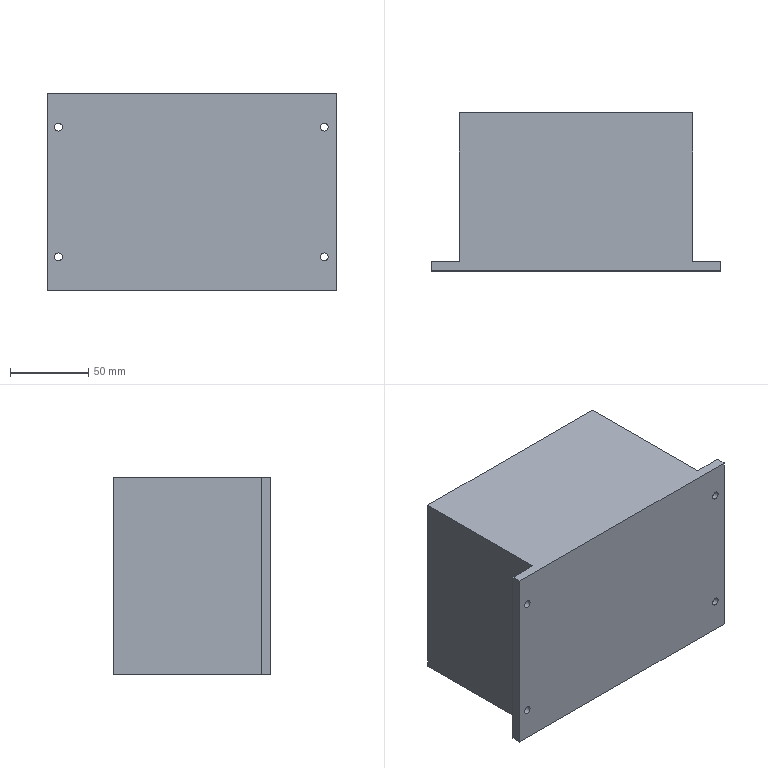Part | STEP file | Inverter | 1 solid | 14 faces | box 185 x 101 x 126 mm | volume 1922919 mm3 | plane 10 | cylinder 4 | commonest cylinder face diameters 5 x4
STEP:
#1=CARTESIAN_POINT('',(0.,0.,0.));
#2=DIRECTION('',(0.,0.,1.));
#3=DIRECTION('',(1.,0.,0.));
#4=AXIS2_PLACEMENT_3D('',#1,#2,#3);
#5=CARTESIAN_POINT('',(-110.145,6.,92.15));
#6=VERTEX_POINT('',#5);
#7=CARTESIAN_POINT('',(-110.145,0.,92.15));
#8=VERTEX_POINT('',#7);
#9=CARTESIAN_POINT('',(-110.145,101.,92.15));
#10=DIRECTION('',(0.,-1.,0.));
#11=VECTOR('',#10,1.);
#12=LINE('',#9,#11);
#13=CARTESIAN_POINT('',(-110.145,101.,-33.85));
#14=DIRECTION('',(1.,0.,0.));
#15=DIRECTION('',(0.,0.,-1.));
#16=AXIS2_PLACEMENT_3D('',#13,#14,#15);
#17=PLANE('',#16);
#18=CARTESIAN_POINT('',(-126.,0.));
#19=DIRECTION('',(0.,-1.));
#20=VECTOR('',#19,1.);
#21=LINE('',#18,#20);
#22=(GEOMETRIC_REPRESENTATION_CONTEXT(2)PARAMETRIC_REPRESENTATION_CONTEXT()REPRESENTATION_CONTEXT('',''));
#23=DEFINITIONAL_REPRESENTATION('',(#21),#22);
#24=PCURVE('',#17,#23);
#25=CARTESIAN_POINT('',(-110.145,101.,92.15));
#26=DIRECTION('',(0.,0.,-1.));
#27=DIRECTION('',(-1.,0.,0.));
#28=AXIS2_PLACEMENT_3D('',#25,#26,#27);
#29=PLANE('',#28);
#30=CARTESIAN_POINT('',(0.,0.));
#31=DIRECTION('',(0.,-1.));
#32=VECTOR('',#31,1.);
#33=LINE('',#30,#32);
#34=(GEOMETRIC_REPRESENTATION_CONTEXT(2)PARAMETRIC_REPRESENTATION_CONTEXT()REPRESENTATION_CONTEXT('',''));
#35=DEFINITIONAL_REPRESENTATION('',(#33),#34);
#36=PCURVE('',#29,#35);
#37=SURFACE_CURVE('',#12,(#24,#36),.PCURVE_S1.);
#38=EDGE_CURVE('',#6,#8,#37,.T.);
#39=ORIENTED_EDGE('',*,*,#38,.F.);
#40=CARTESIAN_POINT('',(-110.145,6.,-33.85));
#41=VERTEX_POINT('',#40);
#42=CARTESIAN_POINT('',(-110.145,6.,-33.85));
#43=DIRECTION('',(0.,0.,-1.));
#44=VECTOR('',#43,1.);
#45=LINE('',#42,#44);
#46=CARTESIAN_POINT('',(0.,-95.));
#47=DIRECTION('',(1.,0.));
#48=VECTOR('',#47,1.);
#49=LINE('',#46,#48);
#50=(GEOMETRIC_REPRESENTATION_CONTEXT(2)PARAMETRIC_REPRESENTATION_CONTEXT()REPRESENTATION_CONTEXT('',''));
#51=DEFINITIONAL_REPRESENTATION('',(#49),#50);
#52=PCURVE('',#17,#51);
#53=CARTESIAN_POINT('',(-116.411,6.,-33.85));
#54=DIRECTION('',(0.,-1.,0.));
#55=DIRECTION('',(0.,0.,-1.));
#56=AXIS2_PLACEMENT_3D('',#53,#54,#55);
#57=PLANE('',#56);
#58=CARTESIAN_POINT('',(0.,6.266));
#59=DIRECTION('',(1.,0.));
#60=VECTOR('',#59,1.);
#61=LINE('',#58,#60);
#62=(GEOMETRIC_REPRESENTATION_CONTEXT(2)PARAMETRIC_REPRESENTATION_CONTEXT()REPRESENTATION_CONTEXT('',''));
#63=DEFINITIONAL_REPRESENTATION('',(#61),#62);
#64=PCURVE('',#57,#63);
#65=SURFACE_CURVE('',#45,(#52,#64),.PCURVE_S1.);
#66=EDGE_CURVE('',#6,#41,#65,.T.);
#67=ORIENTED_EDGE('',*,*,#66,.T.);
#68=CARTESIAN_POINT('',(-110.145,0.,-33.85));
#69=VERTEX_POINT('',#68);
#70=CARTESIAN_POINT('',(-110.145,101.,-33.85));
#71=DIRECTION('',(0.,-1.,0.));
#72=VECTOR('',#71,1.);
#73=LINE('',#70,#72);
#74=CARTESIAN_POINT('',(0.,0.));
#75=DIRECTION('',(0.,-1.));
#76=VECTOR('',#75,1.);
#77=LINE('',#74,#76);
#78=(GEOMETRIC_REPRESENTATION_CONTEXT(2)PARAMETRIC_REPRESENTATION_CONTEXT()REPRESENTATION_CONTEXT('',''));
#79=DEFINITIONAL_REPRESENTATION('',(#77),#78);
#80=PCURVE('',#17,#79);
#81=CARTESIAN_POINT('',(-110.145,101.,-33.85));
#82=DIRECTION('',(0.,0.,1.));
#83=DIRECTION('',(1.,0.,0.));
#84=AXIS2_PLACEMENT_3D('',#81,#82,#83);
#85=PLANE('',#84);
#86=CARTESIAN_POINT('',(0.,0.));
#87=DIRECTION('',(0.,-1.));
#88=VECTOR('',#87,1.);
#89=LINE('',#86,#88);
#90=(GEOMETRIC_REPRESENTATION_CONTEXT(2)PARAMETRIC_REPRESENTATION_CONTEXT()REPRESENTATION_CONTEXT('',''));
#91=DEFINITIONAL_REPRESENTATION('',(#89),#90);
#92=PCURVE('',#85,#91);
#93=SURFACE_CURVE('',#73,(#80,#92),.PCURVE_S1.);
#94=EDGE_CURVE('',#41,#69,#93,.T.);
#95=ORIENTED_EDGE('',*,*,#94,.T.);
#96=CARTESIAN_POINT('',(-110.145,0.,-33.85));
#97=DIRECTION('',(0.,0.,1.));
#98=VECTOR('',#97,1.);
#99=LINE('',#96,#98);
#100=CARTESIAN_POINT('',(0.,-101.));
#101=DIRECTION('',(-1.,0.));
#102=VECTOR('',#101,1.);
#103=LINE('',#100,#102);
#104=(GEOMETRIC_REPRESENTATION_CONTEXT(2)PARAMETRIC_REPRESENTATION_CONTEXT()REPRESENTATION_CONTEXT('',''));
#105=DEFINITIONAL_REPRESENTATION('',(#103),#104);
#106=PCURVE('',#17,#105);
#107=CARTESIAN_POINT('',(0.,0.,0.));
#108=DIRECTION('',(0.,1.,0.));
#109=DIRECTION('',(0.,0.,1.));
#110=AXIS2_PLACEMENT_3D('',#107,#108,#109);
#111=PLANE('',#110);
#112=CARTESIAN_POINT('',(-33.85,-110.145));
#113=DIRECTION('',(1.,0.));
#114=VECTOR('',#113,1.);
#115=LINE('',#112,#114);
#116=(GEOMETRIC_REPRESENTATION_CONTEXT(2)PARAMETRIC_REPRESENTATION_CONTEXT()REPRESENTATION_CONTEXT('',''));
#117=DEFINITIONAL_REPRESENTATION('',(#115),#116);
#118=PCURVE('',#111,#117);
#119=SURFACE_CURVE('',#99,(#106,#118),.PCURVE_S1.);
#120=EDGE_CURVE('',#69,#8,#119,.T.);
#121=ORIENTED_EDGE('',*,*,#120,.T.);
#122=EDGE_LOOP('',(#39,#67,#95,#121));
#123=FACE_BOUND('',#122,.T.);
#124=ADVANCED_FACE('',(#123),#17,.F.);
#125=CARTESIAN_POINT('',(74.855,6.,92.15));
#126=VERTEX_POINT('',#125);
#127=CARTESIAN_POINT('',(74.855,0.,92.15));
#128=VERTEX_POINT('',#127);
#129=CARTESIAN_POINT('',(74.855,101.,92.15));
#130=DIRECTION('',(0.,-1.,0.));
#131=VECTOR('',#130,1.);
#132=LINE('',#129,#131);
#133=CARTESIAN_POINT('',(-185.,0.));
#134=DIRECTION('',(0.,-1.));
#135=VECTOR('',#134,1.);
#136=LINE('',#133,#135);
#137=(GEOMETRIC_REPRESENTATION_CONTEXT(2)PARAMETRIC_REPRESENTATION_CONTEXT()REPRESENTATION_CONTEXT('',''));
#138=DEFINITIONAL_REPRESENTATION('',(#136),#137);
#139=PCURVE('',#29,#138);
#140=CARTESIAN_POINT('',(74.855,101.,-33.85));
#141=DIRECTION('',(-1.,0.,0.));
#142=DIRECTION('',(0.,0.,1.));
#143=AXIS2_PLACEMENT_3D('',#140,#141,#142);
#144=PLANE('',#143);
#145=CARTESIAN_POINT('',(126.,0.));
#146=DIRECTION('',(0.,-1.));
#147=VECTOR('',#146,1.);
#148=LINE('',#145,#147);
#149=(GEOMETRIC_REPRESENTATION_CONTEXT(2)PARAMETRIC_REPRESENTATION_CONTEXT()REPRESENTATION_CONTEXT('',''));
#150=DEFINITIONAL_REPRESENTATION('',(#148),#149);
#151=PCURVE('',#144,#150);
#152=SURFACE_CURVE('',#132,(#139,#151),.PCURVE_S1.);
#153=EDGE_CURVE('',#126,#128,#152,.T.);
#154=ORIENTED_EDGE('',*,*,#153,.F.);
#155=CARTESIAN_POINT('',(56.855,6.,92.15));
#156=VERTEX_POINT('',#155);
#157=CARTESIAN_POINT('',(76.853,6.,92.15));
#158=DIRECTION('',(1.,0.,0.));
#159=VECTOR('',#158,1.);
#160=LINE('',#157,#159);
#161=CARTESIAN_POINT('',(-186.998,-95.));
#162=DIRECTION('',(-1.,0.));
#163=VECTOR('',#162,1.);
#164=LINE('',#161,#163);
#165=(GEOMETRIC_REPRESENTATION_CONTEXT(2)PARAMETRIC_REPRESENTATION_CONTEXT()REPRESENTATION_CONTEXT('',''));
#166=DEFINITIONAL_REPRESENTATION('',(#164),#165);
#167=PCURVE('',#29,#166);
#168=CARTESIAN_POINT('',(76.853,6.,-33.85));
#169=DIRECTION('',(0.,-1.,0.));
#170=DIRECTION('',(1.,0.,0.));
#171=AXIS2_PLACEMENT_3D('',#168,#169,#170);
#172=PLANE('',#171);
#173=CARTESIAN_POINT('',(0.,126.));
#174=DIRECTION('',(1.,0.));
#175=VECTOR('',#174,1.);
#176=LINE('',#173,#175);
#177=(GEOMETRIC_REPRESENTATION_CONTEXT(2)PARAMETRIC_REPRESENTATION_CONTEXT()REPRESENTATION_CONTEXT('',''));
#178=DEFINITIONAL_REPRESENTATION('',(#176),#177);
#179=PCURVE('',#172,#178);
#180=SURFACE_CURVE('',#160,(#167,#179),.PCURVE_S1.);
#181=EDGE_CURVE('',#156,#126,#180,.T.);
#182=ORIENTED_EDGE('',*,*,#181,.F.);
#183=CARTESIAN_POINT('',(56.855,101.,92.15));
#184=VERTEX_POINT('',#183);
#185=CARTESIAN_POINT('',(56.855,105.316,92.15));
#186=DIRECTION('',(0.,-1.,0.));
#187=VECTOR('',#186,1.);
#188=LINE('',#185,#187);
#189=CARTESIAN_POINT('',(-167.,4.316));
#190=DIRECTION('',(0.,-1.));
#191=VECTOR('',#190,1.);
#192=LINE('',#189,#191);
#193=(GEOMETRIC_REPRESENTATION_CONTEXT(2)PARAMETRIC_REPRESENTATION_CONTEXT()REPRESENTATION_CONTEXT('',''));
#194=DEFINITIONAL_REPRESENTATION('',(#192),#193);
#195=PCURVE('',#29,#194);
#196=CARTESIAN_POINT('',(56.855,105.316,-33.85));
#197=DIRECTION('',(-1.,0.,0.));
#198=DIRECTION('',(0.,-1.,0.));
#199=AXIS2_PLACEMENT_3D('',#196,#197,#198);
#200=PLANE('',#199);
#201=CARTESIAN_POINT('',(0.,126.));
#202=DIRECTION('',(1.,0.));
#203=VECTOR('',#202,1.);
#204=LINE('',#201,#203);
#205=(GEOMETRIC_REPRESENTATION_CONTEXT(2)PARAMETRIC_REPRESENTATION_CONTEXT()REPRESENTATION_CONTEXT('',''));
#206=DEFINITIONAL_REPRESENTATION('',(#204),#205);
#207=PCURVE('',#200,#206);
#208=SURFACE_CURVE('',#188,(#195,#207),.PCURVE_S1.);
#209=EDGE_CURVE('',#184,#156,#208,.T.);
#210=ORIENTED_EDGE('',*,*,#209,.F.);
#211=CARTESIAN_POINT('',(-92.145,101.,92.15));
#212=VERTEX_POINT('',#211);
#213=CARTESIAN_POINT('',(-110.145,101.,92.15));
#214=DIRECTION('',(1.,0.,0.));
#215=VECTOR('',#214,1.);
#216=LINE('',#213,#215);
#217=CARTESIAN_POINT('',(0.,0.));
#218=DIRECTION('',(-1.,0.));
#219=VECTOR('',#218,1.);
#220=LINE('',#217,#219);
#221=(GEOMETRIC_REPRESENTATION_CONTEXT(2)PARAMETRIC_REPRESENTATION_CONTEXT()REPRESENTATION_CONTEXT('',''));
#222=DEFINITIONAL_REPRESENTATION('',(#220),#221);
#223=PCURVE('',#29,#222);
#224=CARTESIAN_POINT('',(0.,101.,0.));
#225=DIRECTION('',(0.,1.,0.));
#226=DIRECTION('',(0.,0.,1.));
#227=AXIS2_PLACEMENT_3D('',#224,#225,#226);
#228=PLANE('',#227);
#229=CARTESIAN_POINT('',(92.15,-110.145));
#230=DIRECTION('',(0.,1.));
#231=VECTOR('',#230,1.);
#232=LINE('',#229,#231);
#233=(GEOMETRIC_REPRESENTATION_CONTEXT(2)PARAMETRIC_REPRESENTATION_CONTEXT()REPRESENTATION_CONTEXT('',''));
#234=DEFINITIONAL_REPRESENTATION('',(#232),#233);
#235=PCURVE('',#228,#234);
#236=SURFACE_CURVE('',#216,(#223,#235),.PCURVE_S1.);
#237=EDGE_CURVE('',#212,#184,#236,.T.);
#238=ORIENTED_EDGE('',*,*,#237,.F.);
#239=CARTESIAN_POINT('',(-92.145,6.,92.15));
#240=VERTEX_POINT('',#239);
#241=CARTESIAN_POINT('',(-92.145,101.412,92.15));
#242=DIRECTION('',(0.,1.,0.));
#243=VECTOR('',#242,1.);
#244=LINE('',#241,#243);
#245=CARTESIAN_POINT('',(-18.,0.4121));
#246=DIRECTION('',(0.,1.));
#247=VECTOR('',#246,1.);
#248=LINE('',#245,#247);
#249=(GEOMETRIC_REPRESENTATION_CONTEXT(2)PARAMETRIC_REPRESENTATION_CONTEXT()REPRESENTATION_CONTEXT('',''));
#250=DEFINITIONAL_REPRESENTATION('',(#248),#249);
#251=PCURVE('',#29,#250);
#252=CARTESIAN_POINT('',(-92.145,101.412,-33.85));
#253=DIRECTION('',(1.,0.,0.));
#254=DIRECTION('',(0.,1.,0.));
#255=AXIS2_PLACEMENT_3D('',#252,#253,#254);
#256=PLANE('',#255);
#257=CARTESIAN_POINT('',(0.,126.));
#258=DIRECTION('',(1.,0.));
#259=VECTOR('',#258,1.);
#260=LINE('',#257,#259);
#261=(GEOMETRIC_REPRESENTATION_CONTEXT(2)PARAMETRIC_REPRESENTATION_CONTEXT()REPRESENTATION_CONTEXT('',''));
#262=DEFINITIONAL_REPRESENTATION('',(#260),#261);
#263=PCURVE('',#256,#262);
#264=SURFACE_CURVE('',#244,(#251,#263),.PCURVE_S1.);
#265=EDGE_CURVE('',#240,#212,#264,.T.);
#266=ORIENTED_EDGE('',*,*,#265,.F.);
#267=CARTESIAN_POINT('',(-116.411,6.,92.15));
#268=DIRECTION('',(1.,0.,0.));
#269=VECTOR('',#268,1.);
#270=LINE('',#267,#269);
#271=CARTESIAN_POINT('',(6.266,-95.));
#272=DIRECTION('',(-1.,0.));
#273=VECTOR('',#272,1.);
#274=LINE('',#271,#273);
#275=(GEOMETRIC_REPRESENTATION_CONTEXT(2)PARAMETRIC_REPRESENTATION_CONTEXT()REPRESENTATION_CONTEXT('',''));
#276=DEFINITIONAL_REPRESENTATION('',(#274),#275);
#277=PCURVE('',#29,#276);
#278=CARTESIAN_POINT('',(-126.,0.));
#279=DIRECTION('',(0.,1.));
#280=VECTOR('',#279,1.);
#281=LINE('',#278,#280);
#282=(GEOMETRIC_REPRESENTATION_CONTEXT(2)PARAMETRIC_REPRESENTATION_CONTEXT()REPRESENTATION_CONTEXT('',''));
#283=DEFINITIONAL_REPRESENTATION('',(#281),#282);
#284=PCURVE('',#57,#283);
#285=SURFACE_CURVE('',#270,(#277,#284),.PCURVE_S1.);
#286=EDGE_CURVE('',#6,#240,#285,.T.);
#287=ORIENTED_EDGE('',*,*,#286,.F.);
#288=ORIENTED_EDGE('',*,*,#38,.T.);
#289=CARTESIAN_POINT('',(-110.145,0.,92.15));
#290=DIRECTION('',(1.,0.,0.));
#291=VECTOR('',#290,1.);
#292=LINE('',#289,#291);
#293=CARTESIAN_POINT('',(0.,-101.));
#294=DIRECTION('',(-1.,0.));
#295=VECTOR('',#294,1.);
#296=LINE('',#293,#295);
#297=(GEOMETRIC_REPRESENTATION_CONTEXT(2)PARAMETRIC_REPRESENTATION_CONTEXT()REPRESENTATION_CONTEXT('',''));
#298=DEFINITIONAL_REPRESENTATION('',(#296),#297);
#299=PCURVE('',#29,#298);
#300=CARTESIAN_POINT('',(92.15,-110.145));
#301=DIRECTION('',(0.,1.));
#302=VECTOR('',#301,1.);
#303=LINE('',#300,#302);
#304=(GEOMETRIC_REPRESENTATION_CONTEXT(2)PARAMETRIC_REPRESENTATION_CONTEXT()REPRESENTATION_CONTEXT('',''));
#305=DEFINITIONAL_REPRESENTATION('',(#303),#304);
#306=PCURVE('',#111,#305);
#307=SURFACE_CURVE('',#292,(#299,#306),.PCURVE_S1.);
#308=EDGE_CURVE('',#8,#128,#307,.T.);
#309=ORIENTED_EDGE('',*,*,#308,.T.);
#310=EDGE_LOOP('',(#154,#182,#210,#238,#266,#287,#288,#309));
#311=FACE_BOUND('',#310,.T.);
#312=ADVANCED_FACE('',(#311),#29,.F.);
#313=CARTESIAN_POINT('',(74.855,6.,-33.85));
#314=VERTEX_POINT('',#313);
#315=CARTESIAN_POINT('',(74.855,0.,-33.85));
#316=VERTEX_POINT('',#315);
#317=CARTESIAN_POINT('',(74.855,101.,-33.85));
#318=DIRECTION('',(0.,-1.,0.));
#319=VECTOR('',#318,1.);
#320=LINE('',#317,#319);
#321=CARTESIAN_POINT('',(0.,0.));
#322=DIRECTION('',(0.,-1.));
#323=VECTOR('',#322,1.);
#324=LINE('',#321,#323);
#325=(GEOMETRIC_REPRESENTATION_CONTEXT(2)PARAMETRIC_REPRESENTATION_CONTEXT()REPRESENTATION_CONTEXT('',''));
#326=DEFINITIONAL_REPRESENTATION('',(#324),#325);
#327=PCURVE('',#144,#326);
#328=CARTESIAN_POINT('',(185.,0.));
#329=DIRECTION('',(0.,-1.));
#330=VECTOR('',#329,1.);
#331=LINE('',#328,#330);
#332=(GEOMETRIC_REPRESENTATION_CONTEXT(2)PARAMETRIC_REPRESENTATION_CONTEXT()REPRESENTATION_CONTEXT('',''));
#333=DEFINITIONAL_REPRESENTATION('',(#331),#332);
#334=PCURVE('',#85,#333);
#335=SURFACE_CURVE('',#320,(#327,#334),.PCURVE_S1.);
#336=EDGE_CURVE('',#314,#316,#335,.T.);
#337=ORIENTED_EDGE('',*,*,#336,.F.);
#338=CARTESIAN_POINT('',(74.855,6.,-33.85));
#339=DIRECTION('',(0.,0.,1.));
#340=VECTOR('',#339,1.);
#341=LINE('',#338,#340);
#342=CARTESIAN_POINT('',(0.,-95.));
#343=DIRECTION('',(1.,0.));
#344=VECTOR('',#343,1.);
#345=LINE('',#342,#344);
#346=(GEOMETRIC_REPRESENTATION_CONTEXT(2)PARAMETRIC_REPRESENTATION_CONTEXT()REPRESENTATION_CONTEXT('',''));
#347=DEFINITIONAL_REPRESENTATION('',(#345),#346);
#348=PCURVE('',#144,#347);
#349=CARTESIAN_POINT('',(-1.998,0.));
#350=DIRECTION('',(0.,1.));
#351=VECTOR('',#350,1.);
#352=LINE('',#349,#351);
#353=(GEOMETRIC_REPRESENTATION_CONTEXT(2)PARAMETRIC_REPRESENTATION_CONTEXT()REPRESENTATION_CONTEXT('',''));
#354=DEFINITIONAL_REPRESENTATION('',(#352),#353);
#355=PCURVE('',#172,#354);
#356=SURFACE_CURVE('',#341,(#348,#355),.PCURVE_S1.);
#357=EDGE_CURVE('',#314,#126,#356,.T.);
#358=ORIENTED_EDGE('',*,*,#357,.T.);
#359=ORIENTED_EDGE('',*,*,#153,.T.);
#360=CARTESIAN_POINT('',(74.855,0.,-33.85));
#361=DIRECTION('',(0.,0.,-1.));
#362=VECTOR('',#361,1.);
#363=LINE('',#360,#362);
#364=CARTESIAN_POINT('',(0.,-101.));
#365=DIRECTION('',(-1.,0.));
#366=VECTOR('',#365,1.);
#367=LINE('',#364,#366);
#368=(GEOMETRIC_REPRESENTATION_CONTEXT(2)PARAMETRIC_REPRESENTATION_CONTEXT()REPRESENTATION_CONTEXT('',''));
#369=DEFINITIONAL_REPRESENTATION('',(#367),#368);
#370=PCURVE('',#144,#369);
#371=CARTESIAN_POINT('',(-33.85,74.855));
#372=DIRECTION('',(-1.,0.));
#373=VECTOR('',#372,1.);
#374=LINE('',#371,#373);
#375=(GEOMETRIC_REPRESENTATION_CONTEXT(2)PARAMETRIC_REPRESENTATION_CONTEXT()REPRESENTATION_CONTEXT('',''));
#376=DEFINITIONAL_REPRESENTATION('',(#374),#375);
#377=PCURVE('',#111,#376);
#378=SURFACE_CURVE('',#363,(#370,#377),.PCURVE_S1.);
#379=EDGE_CURVE('',#128,#316,#378,.T.);
#380=ORIENTED_EDGE('',*,*,#379,.T.);
#381=EDGE_LOOP('',(#337,#358,#359,#380));
#382=FACE_BOUND('',#381,.T.);
#383=ADVANCED_FACE('',(#382),#144,.F.);
#384=CARTESIAN_POINT('',(56.855,101.,-33.85));
#385=VERTEX_POINT('',#384);
#386=CARTESIAN_POINT('',(56.855,6.,-33.85));
#387=VERTEX_POINT('',#386);
#388=CARTESIAN_POINT('',(56.855,105.316,-33.85));
#389=DIRECTION('',(0.,-1.,0.));
#390=VECTOR('',#389,1.);
#391=LINE('',#388,#390);
#392=CARTESIAN_POINT('',(167.,4.316));
#393=DIRECTION('',(0.,-1.));
#394=VECTOR('',#393,1.);
#395=LINE('',#392,#394);
#396=(GEOMETRIC_REPRESENTATION_CONTEXT(2)PARAMETRIC_REPRESENTATION_CONTEXT()REPRESENTATION_CONTEXT('',''));
#397=DEFINITIONAL_REPRESENTATION('',(#395),#396);
#398=PCURVE('',#85,#397);
#399=CARTESIAN_POINT('',(0.,0.));
#400=DIRECTION('',(1.,0.));
#401=VECTOR('',#400,1.);
#402=LINE('',#399,#401);
#403=(GEOMETRIC_REPRESENTATION_CONTEXT(2)PARAMETRIC_REPRESENTATION_CONTEXT()REPRESENTATION_CONTEXT('',''));
#404=DEFINITIONAL_REPRESENTATION('',(#402),#403);
#405=PCURVE('',#200,#404);
#406=SURFACE_CURVE('',#391,(#398,#405),.PCURVE_S1.);
#407=EDGE_CURVE('',#385,#387,#406,.T.);
#408=ORIENTED_EDGE('',*,*,#407,.T.);
#409=CARTESIAN_POINT('',(76.853,6.,-33.85));
#410=DIRECTION('',(1.,0.,0.));
#411=VECTOR('',#410,1.);
#412=LINE('',#409,#411);
#413=CARTESIAN_POINT('',(186.998,-95.));
#414=DIRECTION('',(1.,0.));
#415=VECTOR('',#414,1.);
#416=LINE('',#413,#415);
#417=(GEOMETRIC_REPRESENTATION_CONTEXT(2)PARAMETRIC_REPRESENTATION_CONTEXT()REPRESENTATION_CONTEXT('',''));
#418=DEFINITIONAL_REPRESENTATION('',(#416),#417);
#419=PCURVE('',#85,#418);
#420=CARTESIAN_POINT('',(0.,0.));
#421=DIRECTION('',(1.,0.));
#422=VECTOR('',#421,1.);
#423=LINE('',#420,#422);
#424=(GEOMETRIC_REPRESENTATION_CONTEXT(2)PARAMETRIC_REPRESENTATION_CONTEXT()REPRESENTATION_CONTEXT('',''));
#425=DEFINITIONAL_REPRESENTATION('',(#423),#424);
#426=PCURVE('',#172,#425);
#427=SURFACE_CURVE('',#412,(#419,#426),.PCURVE_S1.);
#428=EDGE_CURVE('',#387,#314,#427,.T.);
#429=ORIENTED_EDGE('',*,*,#428,.T.);
#430=ORIENTED_EDGE('',*,*,#336,.T.);
#431=CARTESIAN_POINT('',(-110.145,0.,-33.85));
#432=DIRECTION('',(-1.,0.,0.));
#433=VECTOR('',#432,1.);
#434=LINE('',#431,#433);
#435=CARTESIAN_POINT('',(0.,-101.));
#436=DIRECTION('',(-1.,0.));
#437=VECTOR('',#436,1.);
#438=LINE('',#435,#437);
#439=(GEOMETRIC_REPRESENTATION_CONTEXT(2)PARAMETRIC_REPRESENTATION_CONTEXT()REPRESENTATION_CONTEXT('',''));
#440=DEFINITIONAL_REPRESENTATION('',(#438),#439);
#441=PCURVE('',#85,#440);
#442=CARTESIAN_POINT('',(-33.85,-110.145));
#443=DIRECTION('',(0.,-1.));
#444=VECTOR('',#443,1.);
#445=LINE('',#442,#444);
#446=(GEOMETRIC_REPRESENTATION_CONTEXT(2)PARAMETRIC_REPRESENTATION_CONTEXT()REPRESENTATION_CONTEXT('',''));
#447=DEFINITIONAL_REPRESENTATION('',(#445),#446);
#448=PCURVE('',#111,#447);
#449=SURFACE_CURVE('',#434,(#441,#448),.PCURVE_S1.);
#450=EDGE_CURVE('',#316,#69,#449,.T.);
#451=ORIENTED_EDGE('',*,*,#450,.T.);
#452=ORIENTED_EDGE('',*,*,#94,.F.);
#453=CARTESIAN_POINT('',(-92.145,6.,-33.85));
#454=VERTEX_POINT('',#453);
#455=CARTESIAN_POINT('',(-116.411,6.,-33.85));
#456=DIRECTION('',(1.,0.,0.));
#457=VECTOR('',#456,1.);
#458=LINE('',#455,#457);
#459=CARTESIAN_POINT('',(-6.266,-95.));
#460=DIRECTION('',(1.,0.));
#461=VECTOR('',#460,1.);
#462=LINE('',#459,#461);
#463=(GEOMETRIC_REPRESENTATION_CONTEXT(2)PARAMETRIC_REPRESENTATION_CONTEXT()REPRESENTATION_CONTEXT('',''));
#464=DEFINITIONAL_REPRESENTATION('',(#462),#463);
#465=PCURVE('',#85,#464);
#466=CARTESIAN_POINT('',(0.,0.));
#467=DIRECTION('',(0.,1.));
#468=VECTOR('',#467,1.);
#469=LINE('',#466,#468);
#470=(GEOMETRIC_REPRESENTATION_CONTEXT(2)PARAMETRIC_REPRESENTATION_CONTEXT()REPRESENTATION_CONTEXT('',''));
#471=DEFINITIONAL_REPRESENTATION('',(#469),#470);
#472=PCURVE('',#57,#471);
#473=SURFACE_CURVE('',#458,(#465,#472),.PCURVE_S1.);
#474=EDGE_CURVE('',#41,#454,#473,.T.);
#475=ORIENTED_EDGE('',*,*,#474,.T.);
#476=CARTESIAN_POINT('',(-92.145,101.,-33.85));
#477=VERTEX_POINT('',#476);
#478=CARTESIAN_POINT('',(-92.145,101.412,-33.85));
#479=DIRECTION('',(0.,1.,0.));
#480=VECTOR('',#479,1.);
#481=LINE('',#478,#480);
#482=CARTESIAN_POINT('',(18.,0.4121));
#483=DIRECTION('',(0.,1.));
#484=VECTOR('',#483,1.);
#485=LINE('',#482,#484);
#486=(GEOMETRIC_REPRESENTATION_CONTEXT(2)PARAMETRIC_REPRESENTATION_CONTEXT()REPRESENTATION_CONTEXT('',''));
#487=DEFINITIONAL_REPRESENTATION('',(#485),#486);
#488=PCURVE('',#85,#487);
#489=CARTESIAN_POINT('',(0.,0.));
#490=DIRECTION('',(1.,0.));
#491=VECTOR('',#490,1.);
#492=LINE('',#489,#491);
#493=(GEOMETRIC_REPRESENTATION_CONTEXT(2)PARAMETRIC_REPRESENTATION_CONTEXT()REPRESENTATION_CONTEXT('',''));
#494=DEFINITIONAL_REPRESENTATION('',(#492),#493);
#495=PCURVE('',#256,#494);
#496=SURFACE_CURVE('',#481,(#488,#495),.PCURVE_S1.);
#497=EDGE_CURVE('',#454,#477,#496,.T.);
#498=ORIENTED_EDGE('',*,*,#497,.T.);
#499=CARTESIAN_POINT('',(-110.145,101.,-33.85));
#500=DIRECTION('',(-1.,0.,0.));
#501=VECTOR('',#500,1.);
#502=LINE('',#499,#501);
#503=CARTESIAN_POINT('',(0.,0.));
#504=DIRECTION('',(-1.,0.));
#505=VECTOR('',#504,1.);
#506=LINE('',#503,#505);
#507=(GEOMETRIC_REPRESENTATION_CONTEXT(2)PARAMETRIC_REPRESENTATION_CONTEXT()REPRESENTATION_CONTEXT('',''));
#508=DEFINITIONAL_REPRESENTATION('',(#506),#507);
#509=PCURVE('',#85,#508);
#510=CARTESIAN_POINT('',(-33.85,-110.145));
#511=DIRECTION('',(0.,-1.));
#512=VECTOR('',#511,1.);
#513=LINE('',#510,#512);
#514=(GEOMETRIC_REPRESENTATION_CONTEXT(2)PARAMETRIC_REPRESENTATION_CONTEXT()REPRESENTATION_CONTEXT('',''));
#515=DEFINITIONAL_REPRESENTATION('',(#513),#514);
#516=PCURVE('',#228,#515);
#517=SURFACE_CURVE('',#502,(#509,#516),.PCURVE_S1.);
#518=EDGE_CURVE('',#385,#477,#517,.T.);
#519=ORIENTED_EDGE('',*,*,#518,.F.);
#520=EDGE_LOOP('',(#408,#429,#430,#451,#452,#475,#498,#519));
#521=FACE_BOUND('',#520,.T.);
#522=ADVANCED_FACE('',(#521),#85,.F.);
#523=CARTESIAN_POINT('',(56.855,101.,0.));
#524=DIRECTION('',(0.,0.,1.));
#525=VECTOR('',#524,1.);
#526=LINE('',#523,#525);
#527=CARTESIAN_POINT('',(0.,56.855));
#528=DIRECTION('',(1.,0.));
#529=VECTOR('',#528,1.);
#530=LINE('',#527,#529);
#531=(GEOMETRIC_REPRESENTATION_CONTEXT(2)PARAMETRIC_REPRESENTATION_CONTEXT()REPRESENTATION_CONTEXT('',''));
#532=DEFINITIONAL_REPRESENTATION('',(#530),#531);
#533=PCURVE('',#228,#532);
#534=CARTESIAN_POINT('',(4.316,33.85));
#535=DIRECTION('',(0.,1.));
#536=VECTOR('',#535,1.);
#537=LINE('',#534,#536);
#538=(GEOMETRIC_REPRESENTATION_CONTEXT(2)PARAMETRIC_REPRESENTATION_CONTEXT()REPRESENTATION_CONTEXT('',''));
#539=DEFINITIONAL_REPRESENTATION('',(#537),#538);
#540=PCURVE('',#200,#539);
#541=SURFACE_CURVE('',#526,(#533,#540),.PCURVE_S1.);
#542=EDGE_CURVE('',#385,#184,#541,.T.);
#543=ORIENTED_EDGE('',*,*,#542,.F.);
#544=ORIENTED_EDGE('',*,*,#518,.T.);
#545=CARTESIAN_POINT('',(-92.145,101.,0.));
#546=DIRECTION('',(0.,0.,-1.));
#547=VECTOR('',#546,1.);
#548=LINE('',#545,#547);
#549=CARTESIAN_POINT('',(0.,-92.145));
#550=DIRECTION('',(-1.,0.));
#551=VECTOR('',#550,1.);
#552=LINE('',#549,#551);
#553=(GEOMETRIC_REPRESENTATION_CONTEXT(2)PARAMETRIC_REPRESENTATION_CONTEXT()REPRESENTATION_CONTEXT('',''));
#554=DEFINITIONAL_REPRESENTATION('',(#552),#553);
#555=PCURVE('',#228,#554);
#556=CARTESIAN_POINT('',(-0.4121,33.85));
#557=DIRECTION('',(0.,-1.));
#558=VECTOR('',#557,1.);
#559=LINE('',#556,#558);
#560=(GEOMETRIC_REPRESENTATION_CONTEXT(2)PARAMETRIC_REPRESENTATION_CONTEXT()REPRESENTATION_CONTEXT('',''));
#561=DEFINITIONAL_REPRESENTATION('',(#559),#560);
#562=PCURVE('',#256,#561);
#563=SURFACE_CURVE('',#548,(#555,#562),.PCURVE_S1.);
#564=EDGE_CURVE('',#212,#477,#563,.T.);
#565=ORIENTED_EDGE('',*,*,#564,.F.);
#566=ORIENTED_EDGE('',*,*,#237,.T.);
#567=EDGE_LOOP('',(#543,#544,#565,#566));
#568=FACE_BOUND('',#567,.T.);
#569=ADVANCED_FACE('',(#568),#228,.T.);
#570=CARTESIAN_POINT('',(66.912,0.,73.15));
#571=VERTEX_POINT('',#570);
#572=CARTESIAN_POINT('',(66.912,0.,70.65));
#573=DIRECTION('',(0.,1.,0.));
#574=DIRECTION('',(0.,0.,1.));
#575=AXIS2_PLACEMENT_3D('',#572,#573,#574);
#576=CIRCLE('',#575,2.5);
#577=CARTESIAN_POINT('',(70.65,66.912));
#578=DIRECTION('',(1.,0.));
#579=AXIS2_PLACEMENT_2D('',#577,#578);
#580=CIRCLE('',#579,2.5);
#581=(GEOMETRIC_REPRESENTATION_CONTEXT(2)PARAMETRIC_REPRESENTATION_CONTEXT()REPRESENTATION_CONTEXT('',''));
#582=DEFINITIONAL_REPRESENTATION('',(#580),#581);
#583=PCURVE('',#111,#582);
#584=CARTESIAN_POINT('',(66.912,-4.,70.65));
#585=DIRECTION('',(0.,1.,0.));
#586=DIRECTION('',(0.,0.,1.));
#587=AXIS2_PLACEMENT_3D('',#584,#585,#586);
#588=CYLINDRICAL_SURFACE('',#587,2.5);
#589=CARTESIAN_POINT('',(0.,4.));
#590=DIRECTION('',(1.,0.));
#591=VECTOR('',#590,1.);
#592=LINE('',#589,#591);
#593=(GEOMETRIC_REPRESENTATION_CONTEXT(2)PARAMETRIC_REPRESENTATION_CONTEXT()REPRESENTATION_CONTEXT('',''));
#594=DEFINITIONAL_REPRESENTATION('',(#592),#593);
#595=PCURVE('',#588,#594);
#596=SURFACE_CURVE('',#576,(#583,#595),.PCURVE_S1.);
#597=EDGE_CURVE('',#571,#571,#596,.T.);
#598=ORIENTED_EDGE('',*,*,#597,.T.);
#599=EDGE_LOOP('',(#598));
#600=FACE_BOUND('',#599,.T.);
#601=CARTESIAN_POINT('',(66.912,0.,-9.85));
#602=VERTEX_POINT('',#601);
#603=CARTESIAN_POINT('',(66.912,0.,-12.35));
#604=DIRECTION('',(0.,1.,0.));
#605=DIRECTION('',(0.,0.,1.));
#606=AXIS2_PLACEMENT_3D('',#603,#604,#605);
#607=CIRCLE('',#606,2.5);
#608=CARTESIAN_POINT('',(-12.35,66.912));
#609=DIRECTION('',(1.,0.));
#610=AXIS2_PLACEMENT_2D('',#608,#609);
#611=CIRCLE('',#610,2.5);
#612=(GEOMETRIC_REPRESENTATION_CONTEXT(2)PARAMETRIC_REPRESENTATION_CONTEXT()REPRESENTATION_CONTEXT('',''));
#613=DEFINITIONAL_REPRESENTATION('',(#611),#612);
#614=PCURVE('',#111,#613);
#615=CARTESIAN_POINT('',(66.912,-4.,-12.35));
#616=DIRECTION('',(0.,1.,0.));
#617=DIRECTION('',(0.,0.,1.));
#618=AXIS2_PLACEMENT_3D('',#615,#616,#617);
#619=CYLINDRICAL_SURFACE('',#618,2.5);
#620=CARTESIAN_POINT('',(0.,4.));
#621=DIRECTION('',(1.,0.));
#622=VECTOR('',#621,1.);
#623=LINE('',#620,#622);
#624=(GEOMETRIC_REPRESENTATION_CONTEXT(2)PARAMETRIC_REPRESENTATION_CONTEXT()REPRESENTATION_CONTEXT('',''));
#625=DEFINITIONAL_REPRESENTATION('',(#623),#624);
#626=PCURVE('',#619,#625);
#627=SURFACE_CURVE('',#607,(#614,#626),.PCURVE_S1.);
#628=EDGE_CURVE('',#602,#602,#627,.T.);
#629=ORIENTED_EDGE('',*,*,#628,.T.);
#630=EDGE_LOOP('',(#629));
#631=FACE_BOUND('',#630,.T.);
#632=CARTESIAN_POINT('',(-103.088,0.,-9.85));
#633=VERTEX_POINT('',#632);
#634=CARTESIAN_POINT('',(-103.088,0.,-12.35));
#635=DIRECTION('',(0.,1.,0.));
#636=DIRECTION('',(0.,0.,1.));
#637=AXIS2_PLACEMENT_3D('',#634,#635,#636);
#638=CIRCLE('',#637,2.5);
#639=CARTESIAN_POINT('',(-12.35,-103.088));
#640=DIRECTION('',(1.,0.));
#641=AXIS2_PLACEMENT_2D('',#639,#640);
#642=CIRCLE('',#641,2.5);
#643=(GEOMETRIC_REPRESENTATION_CONTEXT(2)PARAMETRIC_REPRESENTATION_CONTEXT()REPRESENTATION_CONTEXT('',''));
#644=DEFINITIONAL_REPRESENTATION('',(#642),#643);
#645=PCURVE('',#111,#644);
#646=CARTESIAN_POINT('',(-103.088,-4.,-12.35));
#647=DIRECTION('',(0.,1.,0.));
#648=DIRECTION('',(0.,0.,1.));
#649=AXIS2_PLACEMENT_3D('',#646,#647,#648);
#650=CYLINDRICAL_SURFACE('',#649,2.5);
#651=CARTESIAN_POINT('',(0.,4.));
#652=DIRECTION('',(1.,0.));
#653=VECTOR('',#652,1.);
#654=LINE('',#651,#653);
#655=(GEOMETRIC_REPRESENTATION_CONTEXT(2)PARAMETRIC_REPRESENTATION_CONTEXT()REPRESENTATION_CONTEXT('',''));
#656=DEFINITIONAL_REPRESENTATION('',(#654),#655);
#657=PCURVE('',#650,#656);
#658=SURFACE_CURVE('',#638,(#645,#657),.PCURVE_S1.);
#659=EDGE_CURVE('',#633,#633,#658,.T.);
#660=ORIENTED_EDGE('',*,*,#659,.T.);
#661=EDGE_LOOP('',(#660));
#662=FACE_BOUND('',#661,.T.);
#663=CARTESIAN_POINT('',(-103.088,0.,73.15));
#664=VERTEX_POINT('',#663);
#665=CARTESIAN_POINT('',(-103.088,0.,70.65));
#666=DIRECTION('',(0.,1.,0.));
#667=DIRECTION('',(0.,0.,1.));
#668=AXIS2_PLACEMENT_3D('',#665,#666,#667);
#669=CIRCLE('',#668,2.5);
#670=CARTESIAN_POINT('',(70.65,-103.088));
#671=DIRECTION('',(1.,0.));
#672=AXIS2_PLACEMENT_2D('',#670,#671);
#673=CIRCLE('',#672,2.5);
#674=(GEOMETRIC_REPRESENTATION_CONTEXT(2)PARAMETRIC_REPRESENTATION_CONTEXT()REPRESENTATION_CONTEXT('',''));
#675=DEFINITIONAL_REPRESENTATION('',(#673),#674);
#676=PCURVE('',#111,#675);
#677=CARTESIAN_POINT('',(-103.088,-4.,70.65));
#678=DIRECTION('',(0.,1.,0.));
#679=DIRECTION('',(0.,0.,1.));
#680=AXIS2_PLACEMENT_3D('',#677,#678,#679);
#681=CYLINDRICAL_SURFACE('',#680,2.5);
#682=CARTESIAN_POINT('',(0.,4.));
#683=DIRECTION('',(1.,0.));
#684=VECTOR('',#683,1.);
#685=LINE('',#682,#684);
#686=(GEOMETRIC_REPRESENTATION_CONTEXT(2)PARAMETRIC_REPRESENTATION_CONTEXT()REPRESENTATION_CONTEXT('',''));
#687=DEFINITIONAL_REPRESENTATION('',(#685),#686);
#688=PCURVE('',#681,#687);
#689=SURFACE_CURVE('',#669,(#676,#688),.PCURVE_S1.);
#690=EDGE_CURVE('',#664,#664,#689,.T.);
#691=ORIENTED_EDGE('',*,*,#690,.T.);
#692=EDGE_LOOP('',(#691));
#693=FACE_BOUND('',#692,.T.);
#694=ORIENTED_EDGE('',*,*,#120,.F.);
#695=ORIENTED_EDGE('',*,*,#450,.F.);
#696=ORIENTED_EDGE('',*,*,#379,.F.);
#697=ORIENTED_EDGE('',*,*,#308,.F.);
#698=EDGE_LOOP('',(#694,#695,#696,#697));
#699=FACE_BOUND('',#698,.T.);
#700=ADVANCED_FACE('',(#600,#631,#662,#693,#699),#111,.F.);
#701=CARTESIAN_POINT('',(-103.088,6.,-9.85));
#702=VERTEX_POINT('',#701);
#703=CARTESIAN_POINT('',(-103.088,6.,-12.35));
#704=DIRECTION('',(0.,1.,0.));
#705=DIRECTION('',(0.,0.,1.));
#706=AXIS2_PLACEMENT_3D('',#703,#704,#705);
#707=CIRCLE('',#706,2.5);
#708=CARTESIAN_POINT('',(-24.,13.323));
#709=CARTESIAN_POINT('',(-24.,17.653));
#710=CARTESIAN_POINT('',(-20.25,15.488));
#711=CARTESIAN_POINT('',(-16.5,13.323));
#712=CARTESIAN_POINT('',(-20.25,11.158));
#713=CARTESIAN_POINT('',(-24.,8.993));
#714=CARTESIAN_POINT('',(-24.,13.323));
#715=(BOUNDED_CURVE()B_SPLINE_CURVE(2,(#708,#709,#710,#711,#712,#713,#714),.UNSPECIFIED.,.T.,.F.)B_SPLINE_CURVE_WITH_KNOTS((1,2,2,2,2,1),(-2.094,0.,2.094,4.189,6.283,8.378),.UNSPECIFIED.)CURVE()GEOMETRIC_REPRESENTATION_ITEM()RATIONAL_B_SPLINE_CURVE((1.,0.5,1.,0.5,1.,0.5,1.))REPRESENTATION_ITEM(''));
#716=(GEOMETRIC_REPRESENTATION_CONTEXT(2)PARAMETRIC_REPRESENTATION_CONTEXT()REPRESENTATION_CONTEXT('',''));
#717=DEFINITIONAL_REPRESENTATION('',(#715),#716);
#718=PCURVE('',#57,#717);
#719=CARTESIAN_POINT('',(0.,10.));
#720=DIRECTION('',(1.,0.));
#721=VECTOR('',#720,1.);
#722=LINE('',#719,#721);
#723=(GEOMETRIC_REPRESENTATION_CONTEXT(2)PARAMETRIC_REPRESENTATION_CONTEXT()REPRESENTATION_CONTEXT('',''));
#724=DEFINITIONAL_REPRESENTATION('',(#722),#723);
#725=PCURVE('',#650,#724);
#726=SURFACE_CURVE('',#707,(#718,#725),.PCURVE_S1.);
#727=EDGE_CURVE('',#702,#702,#726,.T.);
#728=ORIENTED_EDGE('',*,*,#727,.F.);
#729=EDGE_LOOP('',(#728));
#730=FACE_BOUND('',#729,.T.);
#731=CARTESIAN_POINT('',(-103.088,6.,73.15));
#732=VERTEX_POINT('',#731);
#733=CARTESIAN_POINT('',(-103.088,6.,70.65));
#734=DIRECTION('',(0.,1.,0.));
#735=DIRECTION('',(0.,0.,1.));
#736=AXIS2_PLACEMENT_3D('',#733,#734,#735);
#737=CIRCLE('',#736,2.5);
#738=CARTESIAN_POINT('',(-107.,13.323));
#739=CARTESIAN_POINT('',(-107.,17.653));
#740=CARTESIAN_POINT('',(-103.25,15.488));
#741=CARTESIAN_POINT('',(-99.5,13.323));
#742=CARTESIAN_POINT('',(-103.25,11.158));
#743=CARTESIAN_POINT('',(-107.,8.993));
#744=CARTESIAN_POINT('',(-107.,13.323));
#745=(BOUNDED_CURVE()B_SPLINE_CURVE(2,(#738,#739,#740,#741,#742,#743,#744),.UNSPECIFIED.,.T.,.F.)B_SPLINE_CURVE_WITH_KNOTS((1,2,2,2,2,1),(-2.094,0.,2.094,4.189,6.283,8.378),.UNSPECIFIED.)CURVE()GEOMETRIC_REPRESENTATION_ITEM()RATIONAL_B_SPLINE_CURVE((1.,0.5,1.,0.5,1.,0.5,1.))REPRESENTATION_ITEM(''));
#746=(GEOMETRIC_REPRESENTATION_CONTEXT(2)PARAMETRIC_REPRESENTATION_CONTEXT()REPRESENTATION_CONTEXT('',''));
#747=DEFINITIONAL_REPRESENTATION('',(#745),#746);
#748=PCURVE('',#57,#747);
#749=CARTESIAN_POINT('',(0.,10.));
#750=DIRECTION('',(1.,0.));
#751=VECTOR('',#750,1.);
#752=LINE('',#749,#751);
#753=(GEOMETRIC_REPRESENTATION_CONTEXT(2)PARAMETRIC_REPRESENTATION_CONTEXT()REPRESENTATION_CONTEXT('',''));
#754=DEFINITIONAL_REPRESENTATION('',(#752),#753);
#755=PCURVE('',#681,#754);
#756=SURFACE_CURVE('',#737,(#748,#755),.PCURVE_S1.);
#757=EDGE_CURVE('',#732,#732,#756,.T.);
#758=ORIENTED_EDGE('',*,*,#757,.F.);
#759=EDGE_LOOP('',(#758));
#760=FACE_BOUND('',#759,.T.);
#761=ORIENTED_EDGE('',*,*,#286,.T.);
#762=CARTESIAN_POINT('',(-92.145,6.,-33.85));
#763=DIRECTION('',(0.,0.,1.));
#764=VECTOR('',#763,1.);
#765=LINE('',#762,#764);
#766=CARTESIAN_POINT('',(0.,24.266));
#767=DIRECTION('',(-1.,0.));
#768=VECTOR('',#767,1.);
#769=LINE('',#766,#768);
#770=(GEOMETRIC_REPRESENTATION_CONTEXT(2)PARAMETRIC_REPRESENTATION_CONTEXT()REPRESENTATION_CONTEXT('',''));
#771=DEFINITIONAL_REPRESENTATION('',(#769),#770);
#772=PCURVE('',#57,#771);
#773=CARTESIAN_POINT('',(-95.412,0.));
#774=DIRECTION('',(0.,1.));
#775=VECTOR('',#774,1.);
#776=LINE('',#773,#775);
#777=(GEOMETRIC_REPRESENTATION_CONTEXT(2)PARAMETRIC_REPRESENTATION_CONTEXT()REPRESENTATION_CONTEXT('',''));
#778=DEFINITIONAL_REPRESENTATION('',(#776),#777);
#779=PCURVE('',#256,#778);
#780=SURFACE_CURVE('',#765,(#772,#779),.PCURVE_S1.);
#781=EDGE_CURVE('',#454,#240,#780,.T.);
#782=ORIENTED_EDGE('',*,*,#781,.F.);
#783=ORIENTED_EDGE('',*,*,#474,.F.);
#784=ORIENTED_EDGE('',*,*,#66,.F.);
#785=EDGE_LOOP('',(#761,#782,#783,#784));
#786=FACE_BOUND('',#785,.T.);
#787=ADVANCED_FACE('',(#730,#760,#786),#57,.F.);
#788=ORIENTED_EDGE('',*,*,#564,.T.);
#789=ORIENTED_EDGE('',*,*,#497,.F.);
#790=ORIENTED_EDGE('',*,*,#781,.T.);
#791=ORIENTED_EDGE('',*,*,#265,.T.);
#792=EDGE_LOOP('',(#788,#789,#790,#791));
#793=FACE_BOUND('',#792,.T.);
#794=ADVANCED_FACE('',(#793),#256,.F.);
#795=CARTESIAN_POINT('',(66.912,6.,73.15));
#796=VERTEX_POINT('',#795);
#797=CARTESIAN_POINT('',(66.912,6.,70.65));
#798=DIRECTION('',(0.,1.,0.));
#799=DIRECTION('',(0.,0.,1.));
#800=AXIS2_PLACEMENT_3D('',#797,#798,#799);
#801=CIRCLE('',#800,2.5);
#802=CARTESIAN_POINT('',(-9.941,107.));
#803=CARTESIAN_POINT('',(-5.611,107.));
#804=CARTESIAN_POINT('',(-7.776,103.25));
#805=CARTESIAN_POINT('',(-9.941,99.5));
#806=CARTESIAN_POINT('',(-12.106,103.25));
#807=CARTESIAN_POINT('',(-14.271,107.));
#808=CARTESIAN_POINT('',(-9.941,107.));
#809=(BOUNDED_CURVE()B_SPLINE_CURVE(2,(#802,#803,#804,#805,#806,#807,#808),.UNSPECIFIED.,.T.,.F.)B_SPLINE_CURVE_WITH_KNOTS((1,2,2,2,2,1),(-2.094,0.,2.094,4.189,6.283,8.378),.UNSPECIFIED.)CURVE()GEOMETRIC_REPRESENTATION_ITEM()RATIONAL_B_SPLINE_CURVE((1.,0.5,1.,0.5,1.,0.5,1.))REPRESENTATION_ITEM(''));
#810=(GEOMETRIC_REPRESENTATION_CONTEXT(2)PARAMETRIC_REPRESENTATION_CONTEXT()REPRESENTATION_CONTEXT('',''));
#811=DEFINITIONAL_REPRESENTATION('',(#809),#810);
#812=PCURVE('',#172,#811);
#813=CARTESIAN_POINT('',(0.,10.));
#814=DIRECTION('',(1.,0.));
#815=VECTOR('',#814,1.);
#816=LINE('',#813,#815);
#817=(GEOMETRIC_REPRESENTATION_CONTEXT(2)PARAMETRIC_REPRESENTATION_CONTEXT()REPRESENTATION_CONTEXT('',''));
#818=DEFINITIONAL_REPRESENTATION('',(#816),#817);
#819=PCURVE('',#588,#818);
#820=SURFACE_CURVE('',#801,(#812,#819),.PCURVE_S1.);
#821=EDGE_CURVE('',#796,#796,#820,.T.);
#822=ORIENTED_EDGE('',*,*,#821,.F.);
#823=EDGE_LOOP('',(#822));
#824=FACE_BOUND('',#823,.T.);
#825=CARTESIAN_POINT('',(66.912,6.,-9.85));
#826=VERTEX_POINT('',#825);
#827=CARTESIAN_POINT('',(66.912,6.,-12.35));
#828=DIRECTION('',(0.,1.,0.));
#829=DIRECTION('',(0.,0.,1.));
#830=AXIS2_PLACEMENT_3D('',#827,#828,#829);
#831=CIRCLE('',#830,2.5);
#832=CARTESIAN_POINT('',(-9.941,24.));
#833=CARTESIAN_POINT('',(-5.611,24.));
#834=CARTESIAN_POINT('',(-7.776,20.25));
#835=CARTESIAN_POINT('',(-9.941,16.5));
#836=CARTESIAN_POINT('',(-12.106,20.25));
#837=CARTESIAN_POINT('',(-14.271,24.));
#838=CARTESIAN_POINT('',(-9.941,24.));
#839=(BOUNDED_CURVE()B_SPLINE_CURVE(2,(#832,#833,#834,#835,#836,#837,#838),.UNSPECIFIED.,.T.,.F.)B_SPLINE_CURVE_WITH_KNOTS((1,2,2,2,2,1),(-2.094,0.,2.094,4.189,6.283,8.378),.UNSPECIFIED.)CURVE()GEOMETRIC_REPRESENTATION_ITEM()RATIONAL_B_SPLINE_CURVE((1.,0.5,1.,0.5,1.,0.5,1.))REPRESENTATION_ITEM(''));
#840=(GEOMETRIC_REPRESENTATION_CONTEXT(2)PARAMETRIC_REPRESENTATION_CONTEXT()REPRESENTATION_CONTEXT('',''));
#841=DEFINITIONAL_REPRESENTATION('',(#839),#840);
#842=PCURVE('',#172,#841);
#843=CARTESIAN_POINT('',(0.,10.));
#844=DIRECTION('',(1.,0.));
#845=VECTOR('',#844,1.);
#846=LINE('',#843,#845);
#847=(GEOMETRIC_REPRESENTATION_CONTEXT(2)PARAMETRIC_REPRESENTATION_CONTEXT()REPRESENTATION_CONTEXT('',''));
#848=DEFINITIONAL_REPRESENTATION('',(#846),#847);
#849=PCURVE('',#619,#848);
#850=SURFACE_CURVE('',#831,(#842,#849),.PCURVE_S1.);
#851=EDGE_CURVE('',#826,#826,#850,.T.);
#852=ORIENTED_EDGE('',*,*,#851,.F.);
#853=EDGE_LOOP('',(#852));
#854=FACE_BOUND('',#853,.T.);
#855=ORIENTED_EDGE('',*,*,#428,.F.);
#856=CARTESIAN_POINT('',(56.855,6.,-33.85));
#857=DIRECTION('',(0.,0.,1.));
#858=VECTOR('',#857,1.);
#859=LINE('',#856,#858);
#860=CARTESIAN_POINT('',(-19.998,0.));
#861=DIRECTION('',(0.,1.));
#862=VECTOR('',#861,1.);
#863=LINE('',#860,#862);
#864=(GEOMETRIC_REPRESENTATION_CONTEXT(2)PARAMETRIC_REPRESENTATION_CONTEXT()REPRESENTATION_CONTEXT('',''));
#865=DEFINITIONAL_REPRESENTATION('',(#863),#864);
#866=PCURVE('',#172,#865);
#867=CARTESIAN_POINT('',(99.316,0.));
#868=DIRECTION('',(0.,1.));
#869=VECTOR('',#868,1.);
#870=LINE('',#867,#869);
#871=(GEOMETRIC_REPRESENTATION_CONTEXT(2)PARAMETRIC_REPRESENTATION_CONTEXT()REPRESENTATION_CONTEXT('',''));
#872=DEFINITIONAL_REPRESENTATION('',(#870),#871);
#873=PCURVE('',#200,#872);
#874=SURFACE_CURVE('',#859,(#866,#873),.PCURVE_S1.);
#875=EDGE_CURVE('',#387,#156,#874,.T.);
#876=ORIENTED_EDGE('',*,*,#875,.T.);
#877=ORIENTED_EDGE('',*,*,#181,.T.);
#878=ORIENTED_EDGE('',*,*,#357,.F.);
#879=EDGE_LOOP('',(#855,#876,#877,#878));
#880=FACE_BOUND('',#879,.T.);
#881=ADVANCED_FACE('',(#824,#854,#880),#172,.F.);
#882=ORIENTED_EDGE('',*,*,#542,.T.);
#883=ORIENTED_EDGE('',*,*,#209,.T.);
#884=ORIENTED_EDGE('',*,*,#875,.F.);
#885=ORIENTED_EDGE('',*,*,#407,.F.);
#886=EDGE_LOOP('',(#882,#883,#884,#885));
#887=FACE_BOUND('',#886,.T.);
#888=ADVANCED_FACE('',(#887),#200,.F.);
#889=ORIENTED_EDGE('',*,*,#757,.F.);
#890=CARTESIAN_POINT('',(-103.088,0.,73.15));
#891=CARTESIAN_POINT('',(-103.088,6.,73.15));
#892=B_SPLINE_CURVE_WITH_KNOTS('',1,(#890,#891),.UNSPECIFIED.,.F.,.F.,(2,2),(4.,10.),.PIECEWISE_BEZIER_KNOTS.);
#893=CARTESIAN_POINT('',(0.,0.));
#894=DIRECTION('',(0.,1.));
#895=VECTOR('',#894,1.);
#896=LINE('',#893,#895);
#897=(GEOMETRIC_REPRESENTATION_CONTEXT(2)PARAMETRIC_REPRESENTATION_CONTEXT()REPRESENTATION_CONTEXT('',''));
#898=DEFINITIONAL_REPRESENTATION('',(#896),#897);
#899=PCURVE('',#681,#898);
#900=CARTESIAN_POINT('',(6.283,0.));
#901=DIRECTION('',(0.,1.));
#902=VECTOR('',#901,1.);
#903=LINE('',#900,#902);
#904=(GEOMETRIC_REPRESENTATION_CONTEXT(2)PARAMETRIC_REPRESENTATION_CONTEXT()REPRESENTATION_CONTEXT('',''));
#905=DEFINITIONAL_REPRESENTATION('',(#903),#904);
#906=PCURVE('',#681,#905);
#907=SEAM_CURVE('',#892,(#899,#906),.PCURVE_S1.);
#908=EDGE_CURVE('',#664,#732,#907,.T.);
#909=ORIENTED_EDGE('',*,*,#908,.F.);
#910=ORIENTED_EDGE('',*,*,#690,.T.);
#911=ORIENTED_EDGE('',*,*,#908,.T.);
#912=EDGE_LOOP('',(#889,#909,#910,#911));
#913=FACE_BOUND('',#912,.F.);
#914=ADVANCED_FACE('',(#913),#681,.F.);
#915=ORIENTED_EDGE('',*,*,#727,.F.);
#916=CARTESIAN_POINT('',(-103.088,0.,-9.85));
#917=CARTESIAN_POINT('',(-103.088,6.,-9.85));
#918=B_SPLINE_CURVE_WITH_KNOTS('',1,(#916,#917),.UNSPECIFIED.,.F.,.F.,(2,2),(4.,10.),.PIECEWISE_BEZIER_KNOTS.);
#919=CARTESIAN_POINT('',(0.,0.));
#920=DIRECTION('',(0.,1.));
#921=VECTOR('',#920,1.);
#922=LINE('',#919,#921);
#923=(GEOMETRIC_REPRESENTATION_CONTEXT(2)PARAMETRIC_REPRESENTATION_CONTEXT()REPRESENTATION_CONTEXT('',''));
#924=DEFINITIONAL_REPRESENTATION('',(#922),#923);
#925=PCURVE('',#650,#924);
#926=CARTESIAN_POINT('',(6.283,0.));
#927=DIRECTION('',(0.,1.));
#928=VECTOR('',#927,1.);
#929=LINE('',#926,#928);
#930=(GEOMETRIC_REPRESENTATION_CONTEXT(2)PARAMETRIC_REPRESENTATION_CONTEXT()REPRESENTATION_CONTEXT('',''));
#931=DEFINITIONAL_REPRESENTATION('',(#929),#930);
#932=PCURVE('',#650,#931);
#933=SEAM_CURVE('',#918,(#925,#932),.PCURVE_S1.);
#934=EDGE_CURVE('',#633,#702,#933,.T.);
#935=ORIENTED_EDGE('',*,*,#934,.F.);
#936=ORIENTED_EDGE('',*,*,#659,.T.);
#937=ORIENTED_EDGE('',*,*,#934,.T.);
#938=EDGE_LOOP('',(#915,#935,#936,#937));
#939=FACE_BOUND('',#938,.F.);
#940=ADVANCED_FACE('',(#939),#650,.F.);
#941=ORIENTED_EDGE('',*,*,#851,.F.);
#942=CARTESIAN_POINT('',(66.912,0.,-9.85));
#943=CARTESIAN_POINT('',(66.912,6.,-9.85));
#944=B_SPLINE_CURVE_WITH_KNOTS('',1,(#942,#943),.UNSPECIFIED.,.F.,.F.,(2,2),(4.,10.),.PIECEWISE_BEZIER_KNOTS.);
#945=CARTESIAN_POINT('',(0.,0.));
#946=DIRECTION('',(0.,1.));
#947=VECTOR('',#946,1.);
#948=LINE('',#945,#947);
#949=(GEOMETRIC_REPRESENTATION_CONTEXT(2)PARAMETRIC_REPRESENTATION_CONTEXT()REPRESENTATION_CONTEXT('',''));
#950=DEFINITIONAL_REPRESENTATION('',(#948),#949);
#951=PCURVE('',#619,#950);
#952=CARTESIAN_POINT('',(6.283,0.));
#953=DIRECTION('',(0.,1.));
#954=VECTOR('',#953,1.);
#955=LINE('',#952,#954);
#956=(GEOMETRIC_REPRESENTATION_CONTEXT(2)PARAMETRIC_REPRESENTATION_CONTEXT()REPRESENTATION_CONTEXT('',''));
#957=DEFINITIONAL_REPRESENTATION('',(#955),#956);
#958=PCURVE('',#619,#957);
#959=SEAM_CURVE('',#944,(#951,#958),.PCURVE_S1.);
#960=EDGE_CURVE('',#602,#826,#959,.T.);
#961=ORIENTED_EDGE('',*,*,#960,.F.);
#962=ORIENTED_EDGE('',*,*,#628,.T.);
#963=ORIENTED_EDGE('',*,*,#960,.T.);
#964=EDGE_LOOP('',(#941,#961,#962,#963));
#965=FACE_BOUND('',#964,.F.);
#966=ADVANCED_FACE('',(#965),#619,.F.);
#967=ORIENTED_EDGE('',*,*,#821,.F.);
#968=CARTESIAN_POINT('',(66.912,0.,73.15));
#969=CARTESIAN_POINT('',(66.912,6.,73.15));
#970=B_SPLINE_CURVE_WITH_KNOTS('',1,(#968,#969),.UNSPECIFIED.,.F.,.F.,(2,2),(4.,10.),.PIECEWISE_BEZIER_KNOTS.);
#971=CARTESIAN_POINT('',(0.,0.));
#972=DIRECTION('',(0.,1.));
#973=VECTOR('',#972,1.);
#974=LINE('',#971,#973);
#975=(GEOMETRIC_REPRESENTATION_CONTEXT(2)PARAMETRIC_REPRESENTATION_CONTEXT()REPRESENTATION_CONTEXT('',''));
#976=DEFINITIONAL_REPRESENTATION('',(#974),#975);
#977=PCURVE('',#588,#976);
#978=CARTESIAN_POINT('',(6.283,0.));
#979=DIRECTION('',(0.,1.));
#980=VECTOR('',#979,1.);
#981=LINE('',#978,#980);
#982=(GEOMETRIC_REPRESENTATION_CONTEXT(2)PARAMETRIC_REPRESENTATION_CONTEXT()REPRESENTATION_CONTEXT('',''));
#983=DEFINITIONAL_REPRESENTATION('',(#981),#982);
#984=PCURVE('',#588,#983);
#985=SEAM_CURVE('',#970,(#977,#984),.PCURVE_S1.);
#986=EDGE_CURVE('',#571,#796,#985,.T.);
#987=ORIENTED_EDGE('',*,*,#986,.F.);
#988=ORIENTED_EDGE('',*,*,#597,.T.);
#989=ORIENTED_EDGE('',*,*,#986,.T.);
#990=EDGE_LOOP('',(#967,#987,#988,#989));
#991=FACE_BOUND('',#990,.F.);
#992=ADVANCED_FACE('',(#991),#588,.F.);
#993=CLOSED_SHELL('',(#124,#312,#383,#522,#569,#700,#787,#794,#881,#888,#914,#940,#966,#992));
#994=MANIFOLD_SOLID_BREP('',#993);
#995=(LENGTH_UNIT()NAMED_UNIT(*)SI_UNIT(.MILLI.,.METRE.));
#996=UNCERTAINTY_MEASURE_WITH_UNIT(LENGTH_MEASURE(0.000002),#995,'','');
#997=(NAMED_UNIT(*)PLANE_ANGLE_UNIT()SI_UNIT($,.RADIAN.));
#998=(NAMED_UNIT(*)SI_UNIT($,.STERADIAN.)SOLID_ANGLE_UNIT());
#999=(GEOMETRIC_REPRESENTATION_CONTEXT(3)GLOBAL_UNCERTAINTY_ASSIGNED_CONTEXT((#996))GLOBAL_UNIT_ASSIGNED_CONTEXT((#995,#997,#998))REPRESENTATION_CONTEXT('',''));
#1000=ADVANCED_BREP_SHAPE_REPRESENTATION('',(#4,#994),#999);